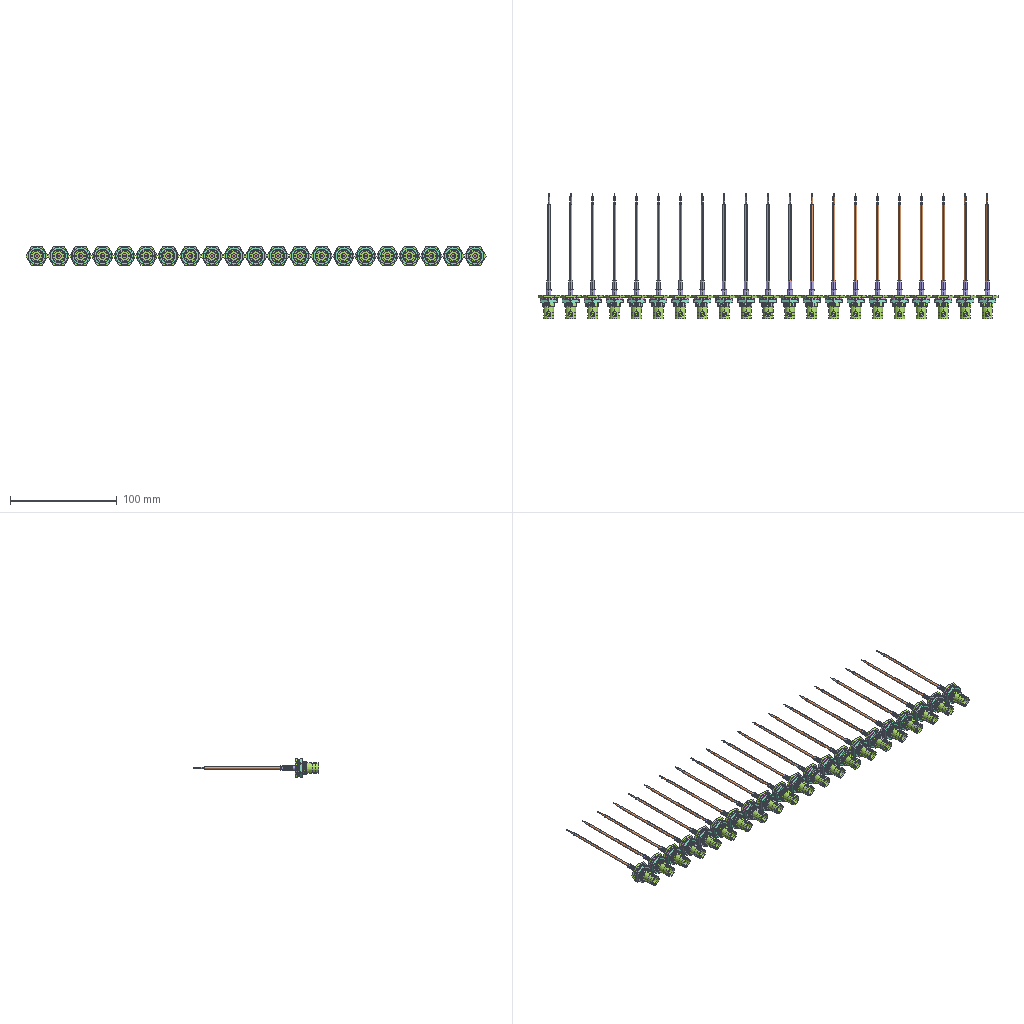Assembly | SolidWorks | 6 different items | 126 placed | box 430 x 117 x 18 mm
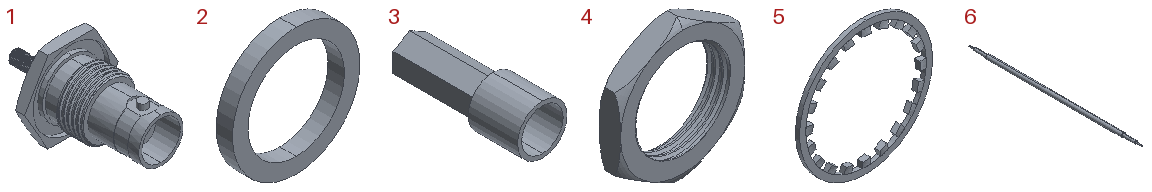Parts list (item | quantity | size | volume | features):
1 | x21 | 20.207 x 31.75 x 17.5 mm | 1414 mm3 | features ICE 8, Helix 2, MirrorPattern 2, Revolution 2, SweepCut 2, CirPattern 1, Extrusion 1, RevCut 1
2 | x21 | 15.6 x 2 x 15.6 mm | 163.551 mm3 | features Extrusion 1
3 | x21 | 5 x 13.4 x 5 mm | 67.021 mm3 | features Extrusion 1, ICE 1, Shell 1
4 | x21 | 16 x 2.75 x 18.475 mm | 281.244 mm3 | features Extrusion 1, Helix 1, RevCut 1, SweepCut 1
5 | x21 | 16 x 0.8028 x 16 mm | 17.966 mm3 | features 3DProfileFeature 10, FillRefSurface 5, CirPattern 1, Extrusion 1, SewRefSurface 1, Thicken 1
6 | x21 | 2.25 x 95.2 x 2.25 mm | 323.59 mm3 | features ICE 4, Extrusion 1
Mates (type | each side: item.copy, entity, surface, feature):
Concentric | 1.1 face cylinder Revolve2 | 2.1 face cylinder Boss-Extrude1
Coincident | 1.1 face plane Cut-Extrude4 | 2.1 face plane Boss-Extrude1
Concentric | 1.1 face cylinder Revolve2 | 5.1 face cylinder Boss-Extrude4
Coincident | 2.1 face plane Boss-Extrude1 | 5.1 vertex
Concentric | 5.1 face cylinder Boss-Extrude4 | 4.1 edge
Coincident | 5.1 vertex | 4.1 face plane Boss-Extrude1
Concentric | 1.1 edge | 6.1 face cylinder Boss-Extrude2
Coincident | 1.1 face plane Boss-Extrude1 | 6.1 face plane Boss-Extrude3
Coincident | 1.1 face plane Boss-Extrude1 | 3.1 face plane Boss-Extrude3
Concentric | 1.1 face cylinder Revolve1 | 3.1 face cylinder Boss-Extrude3